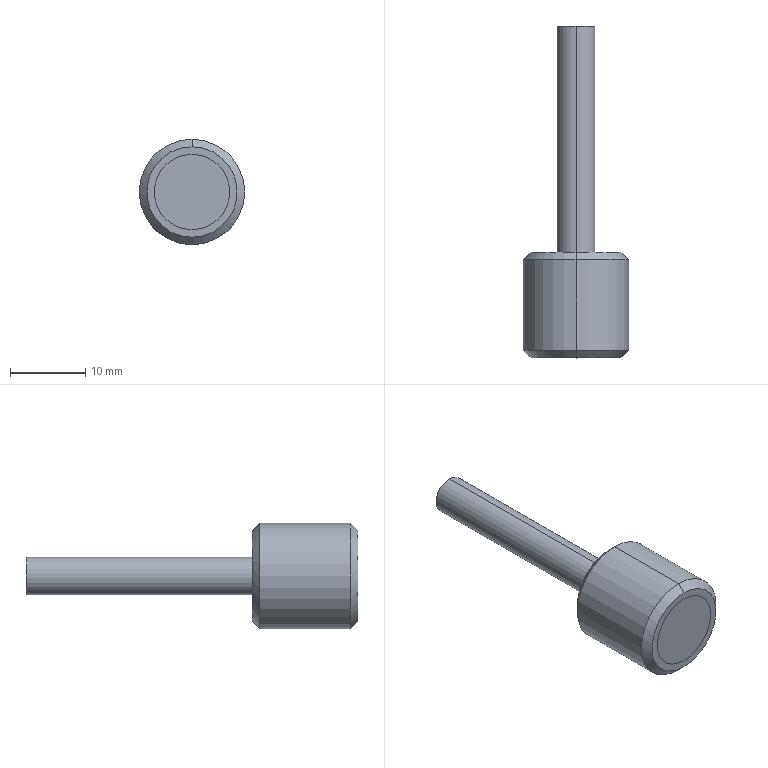Part | STEP file | Pedestal magnet | 2 solids | 18 faces | box 14 x 44 x 14 mm | volume 2702 mm3 | cylinder 8 | plane 6 | cone 4 | commonest cylinder face diameters 10 x4 5 x2 14 x2
STEP:
#1=CARTESIAN_POINT('',(0.,0.,0.));
#2=DIRECTION('',(0.,0.,1.));
#3=DIRECTION('',(1.,0.,0.));
#4=AXIS2_PLACEMENT_3D('',#1,#2,#3);
#5=CARTESIAN_POINT('',(0.,0.,-6.));
#6=VERTEX_POINT('',#5);
#7=CARTESIAN_POINT('',(0.,0.,6.));
#8=VERTEX_POINT('',#7);
#9=CARTESIAN_POINT('',(0.,0.,0.));
#10=DIRECTION('',(0.,-1.,0.));
#11=DIRECTION('',(0.,0.,1.));
#12=AXIS2_PLACEMENT_3D('',#9,#10,#11);
#13=CIRCLE('',#12,6.);
#14=CARTESIAN_POINT('',(0.,1.,0.));
#15=DIRECTION('',(0.,1.,0.));
#16=DIRECTION('',(0.,0.,1.));
#17=AXIS2_PLACEMENT_3D('',#14,#15,#16);
#18=CONICAL_SURFACE('',#17,7.,0.7854);
#19=CARTESIAN_POINT('',(6.283,-1.));
#20=DIRECTION('',(-1.,0.));
#21=VECTOR('',#20,1.);
#22=LINE('',#19,#21);
#23=(GEOMETRIC_REPRESENTATION_CONTEXT(2)PARAMETRIC_REPRESENTATION_CONTEXT()REPRESENTATION_CONTEXT('',''));
#24=DEFINITIONAL_REPRESENTATION('',(#22),#23);
#25=PCURVE('',#18,#24);
#26=CARTESIAN_POINT('',(0.,0.,0.));
#27=DIRECTION('',(0.,1.,0.));
#28=DIRECTION('',(0.,0.,1.));
#29=AXIS2_PLACEMENT_3D('',#26,#27,#28);
#30=PLANE('',#29);
#31=CARTESIAN_POINT('',(6.,0.));
#32=CARTESIAN_POINT('',(6.,-10.392));
#33=CARTESIAN_POINT('',(-3.,-5.196));
#34=CARTESIAN_POINT('',(-12.,0.));
#35=CARTESIAN_POINT('',(-3.,5.196));
#36=CARTESIAN_POINT('',(6.,10.392));
#37=CARTESIAN_POINT('',(6.,0.));
#38=(BOUNDED_CURVE()B_SPLINE_CURVE(2,(#31,#32,#33,#34,#35,#36,#37),.UNSPECIFIED.,.T.,.F.)B_SPLINE_CURVE_WITH_KNOTS((1,2,2,2,2,1),(-2.094,0.,2.094,4.189,6.283,8.378),.UNSPECIFIED.)CURVE()GEOMETRIC_REPRESENTATION_ITEM()RATIONAL_B_SPLINE_CURVE((1.,0.5,1.,0.5,1.,0.5,1.))REPRESENTATION_ITEM(''));
#39=(GEOMETRIC_REPRESENTATION_CONTEXT(2)PARAMETRIC_REPRESENTATION_CONTEXT()REPRESENTATION_CONTEXT('',''));
#40=DEFINITIONAL_REPRESENTATION('',(#38),#39);
#41=PCURVE('',#30,#40);
#42=SURFACE_CURVE('',#13,(#25,#41),.PCURVE_S1.);
#43=EDGE_CURVE('',#6,#8,#42,.T.);
#44=ORIENTED_EDGE('',*,*,#43,.F.);
#45=CARTESIAN_POINT('',(0.,1.,-7.));
#46=VERTEX_POINT('',#45);
#47=CARTESIAN_POINT('',(0.,1.,-7.));
#48=DIRECTION('',(0.,0.7071,-0.7071));
#49=VECTOR('',#48,1.);
#50=LINE('',#47,#49);
#51=CARTESIAN_POINT('',(3.142,0.));
#52=DIRECTION('',(0.,1.));
#53=VECTOR('',#52,1.);
#54=LINE('',#51,#53);
#55=(GEOMETRIC_REPRESENTATION_CONTEXT(2)PARAMETRIC_REPRESENTATION_CONTEXT()REPRESENTATION_CONTEXT('',''));
#56=DEFINITIONAL_REPRESENTATION('',(#54),#55);
#57=PCURVE('',#18,#56);
#58=CARTESIAN_POINT('',(0.,1.,0.));
#59=DIRECTION('',(0.,1.,0.));
#60=DIRECTION('',(0.,0.,1.));
#61=AXIS2_PLACEMENT_3D('',#58,#59,#60);
#62=CONICAL_SURFACE('',#61,7.,0.7854);
#63=CARTESIAN_POINT('',(3.142,0.));
#64=DIRECTION('',(0.,1.));
#65=VECTOR('',#64,1.);
#66=LINE('',#63,#65);
#67=(GEOMETRIC_REPRESENTATION_CONTEXT(2)PARAMETRIC_REPRESENTATION_CONTEXT()REPRESENTATION_CONTEXT('',''));
#68=DEFINITIONAL_REPRESENTATION('',(#66),#67);
#69=PCURVE('',#62,#68);
#70=SURFACE_CURVE('',#50,(#57,#69),.PCURVE_S1.);
#71=EDGE_CURVE('',#6,#46,#70,.T.);
#72=ORIENTED_EDGE('',*,*,#71,.T.);
#73=CARTESIAN_POINT('',(0.,1.,7.));
#74=VERTEX_POINT('',#73);
#75=CARTESIAN_POINT('',(0.,1.,0.));
#76=DIRECTION('',(0.,1.,0.));
#77=DIRECTION('',(0.,0.,1.));
#78=AXIS2_PLACEMENT_3D('',#75,#76,#77);
#79=CIRCLE('',#78,7.);
#80=CARTESIAN_POINT('',(0.,0.));
#81=DIRECTION('',(1.,0.));
#82=VECTOR('',#81,1.);
#83=LINE('',#80,#82);
#84=(GEOMETRIC_REPRESENTATION_CONTEXT(2)PARAMETRIC_REPRESENTATION_CONTEXT()REPRESENTATION_CONTEXT('',''));
#85=DEFINITIONAL_REPRESENTATION('',(#83),#84);
#86=PCURVE('',#18,#85);
#87=CARTESIAN_POINT('',(0.,14.,0.));
#88=DIRECTION('',(0.,-1.,0.));
#89=DIRECTION('',(0.,0.,-1.));
#90=AXIS2_PLACEMENT_3D('',#87,#88,#89);
#91=CYLINDRICAL_SURFACE('',#90,7.);
#92=CARTESIAN_POINT('',(3.142,13.));
#93=DIRECTION('',(-1.,0.));
#94=VECTOR('',#93,1.);
#95=LINE('',#92,#94);
#96=(GEOMETRIC_REPRESENTATION_CONTEXT(2)PARAMETRIC_REPRESENTATION_CONTEXT()REPRESENTATION_CONTEXT('',''));
#97=DEFINITIONAL_REPRESENTATION('',(#95),#96);
#98=PCURVE('',#91,#97);
#99=SURFACE_CURVE('',#79,(#86,#98),.PCURVE_S1.);
#100=EDGE_CURVE('',#74,#46,#99,.T.);
#101=ORIENTED_EDGE('',*,*,#100,.F.);
#102=CARTESIAN_POINT('',(0.,1.,7.));
#103=DIRECTION('',(0.,0.7071,0.7071));
#104=VECTOR('',#103,1.);
#105=LINE('',#102,#104);
#106=CARTESIAN_POINT('',(0.,0.));
#107=DIRECTION('',(0.,1.));
#108=VECTOR('',#107,1.);
#109=LINE('',#106,#108);
#110=(GEOMETRIC_REPRESENTATION_CONTEXT(2)PARAMETRIC_REPRESENTATION_CONTEXT()REPRESENTATION_CONTEXT('',''));
#111=DEFINITIONAL_REPRESENTATION('',(#109),#110);
#112=PCURVE('',#18,#111);
#113=CARTESIAN_POINT('',(6.283,0.));
#114=DIRECTION('',(0.,1.));
#115=VECTOR('',#114,1.);
#116=LINE('',#113,#115);
#117=(GEOMETRIC_REPRESENTATION_CONTEXT(2)PARAMETRIC_REPRESENTATION_CONTEXT()REPRESENTATION_CONTEXT('',''));
#118=DEFINITIONAL_REPRESENTATION('',(#116),#117);
#119=PCURVE('',#62,#118);
#120=SURFACE_CURVE('',#105,(#112,#119),.PCURVE_S1.);
#121=EDGE_CURVE('',#8,#74,#120,.T.);
#122=ORIENTED_EDGE('',*,*,#121,.F.);
#123=EDGE_LOOP('',(#44,#72,#101,#122));
#124=FACE_BOUND('',#123,.T.);
#125=ADVANCED_FACE('',(#124),#18,.T.);
#126=CARTESIAN_POINT('',(0.,14.,6.));
#127=VERTEX_POINT('',#126);
#128=CARTESIAN_POINT('',(0.,14.,-6.));
#129=VERTEX_POINT('',#128);
#130=CARTESIAN_POINT('',(0.,14.,0.));
#131=DIRECTION('',(0.,1.,0.));
#132=DIRECTION('',(0.,0.,1.));
#133=AXIS2_PLACEMENT_3D('',#130,#131,#132);
#134=CIRCLE('',#133,6.);
#135=CARTESIAN_POINT('',(0.,14.,0.));
#136=DIRECTION('',(0.,-1.,0.));
#137=DIRECTION('',(0.,0.,-1.));
#138=AXIS2_PLACEMENT_3D('',#135,#136,#137);
#139=CONICAL_SURFACE('',#138,6.,0.7854);
#140=CARTESIAN_POINT('',(3.142,0.));
#141=DIRECTION('',(-1.,0.));
#142=VECTOR('',#141,1.);
#143=LINE('',#140,#142);
#144=(GEOMETRIC_REPRESENTATION_CONTEXT(2)PARAMETRIC_REPRESENTATION_CONTEXT()REPRESENTATION_CONTEXT('',''));
#145=DEFINITIONAL_REPRESENTATION('',(#143),#144);
#146=PCURVE('',#139,#145);
#147=CARTESIAN_POINT('',(0.,14.,0.));
#148=DIRECTION('',(0.,1.,0.));
#149=DIRECTION('',(0.,0.,1.));
#150=AXIS2_PLACEMENT_3D('',#147,#148,#149);
#151=PLANE('',#150);
#152=CARTESIAN_POINT('',(0.,0.));
#153=DIRECTION('',(1.,0.));
#154=AXIS2_PLACEMENT_2D('',#152,#153);
#155=CIRCLE('',#154,6.);
#156=(GEOMETRIC_REPRESENTATION_CONTEXT(2)PARAMETRIC_REPRESENTATION_CONTEXT()REPRESENTATION_CONTEXT('',''));
#157=DEFINITIONAL_REPRESENTATION('',(#155),#156);
#158=PCURVE('',#151,#157);
#159=SURFACE_CURVE('',#134,(#146,#158),.PCURVE_S1.);
#160=EDGE_CURVE('',#127,#129,#159,.T.);
#161=ORIENTED_EDGE('',*,*,#160,.F.);
#162=CARTESIAN_POINT('',(0.,13.,7.));
#163=VERTEX_POINT('',#162);
#164=CARTESIAN_POINT('',(0.,14.,6.));
#165=DIRECTION('',(0.,-0.7071,0.7071));
#166=VECTOR('',#165,1.);
#167=LINE('',#164,#166);
#168=CARTESIAN_POINT('',(3.142,0.));
#169=DIRECTION('',(0.,1.));
#170=VECTOR('',#169,1.);
#171=LINE('',#168,#170);
#172=(GEOMETRIC_REPRESENTATION_CONTEXT(2)PARAMETRIC_REPRESENTATION_CONTEXT()REPRESENTATION_CONTEXT('',''));
#173=DEFINITIONAL_REPRESENTATION('',(#171),#172);
#174=PCURVE('',#139,#173);
#175=CARTESIAN_POINT('',(0.,14.,0.));
#176=DIRECTION('',(0.,-1.,0.));
#177=DIRECTION('',(0.,0.,-1.));
#178=AXIS2_PLACEMENT_3D('',#175,#176,#177);
#179=CONICAL_SURFACE('',#178,6.,0.7854);
#180=CARTESIAN_POINT('',(3.142,0.));
#181=DIRECTION('',(0.,1.));
#182=VECTOR('',#181,1.);
#183=LINE('',#180,#182);
#184=(GEOMETRIC_REPRESENTATION_CONTEXT(2)PARAMETRIC_REPRESENTATION_CONTEXT()REPRESENTATION_CONTEXT('',''));
#185=DEFINITIONAL_REPRESENTATION('',(#183),#184);
#186=PCURVE('',#179,#185);
#187=SURFACE_CURVE('',#167,(#174,#186),.PCURVE_S1.);
#188=EDGE_CURVE('',#127,#163,#187,.T.);
#189=ORIENTED_EDGE('',*,*,#188,.T.);
#190=CARTESIAN_POINT('',(0.,13.,-7.));
#191=VERTEX_POINT('',#190);
#192=CARTESIAN_POINT('',(0.,13.,0.));
#193=DIRECTION('',(0.,-1.,0.));
#194=DIRECTION('',(0.,0.,1.));
#195=AXIS2_PLACEMENT_3D('',#192,#193,#194);
#196=CIRCLE('',#195,7.);
#197=CARTESIAN_POINT('',(-3.142,1.));
#198=DIRECTION('',(1.,0.));
#199=VECTOR('',#198,1.);
#200=LINE('',#197,#199);
#201=(GEOMETRIC_REPRESENTATION_CONTEXT(2)PARAMETRIC_REPRESENTATION_CONTEXT()REPRESENTATION_CONTEXT('',''));
#202=DEFINITIONAL_REPRESENTATION('',(#200),#201);
#203=PCURVE('',#139,#202);
#204=CARTESIAN_POINT('',(-3.142,1.));
#205=DIRECTION('',(1.,0.));
#206=VECTOR('',#205,1.);
#207=LINE('',#204,#206);
#208=(GEOMETRIC_REPRESENTATION_CONTEXT(2)PARAMETRIC_REPRESENTATION_CONTEXT()REPRESENTATION_CONTEXT('',''));
#209=DEFINITIONAL_REPRESENTATION('',(#207),#208);
#210=PCURVE('',#91,#209);
#211=SURFACE_CURVE('',#196,(#203,#210),.PCURVE_S1.);
#212=EDGE_CURVE('',#191,#163,#211,.T.);
#213=ORIENTED_EDGE('',*,*,#212,.F.);
#214=CARTESIAN_POINT('',(0.,14.,-6.));
#215=DIRECTION('',(0.,-0.7071,-0.7071));
#216=VECTOR('',#215,1.);
#217=LINE('',#214,#216);
#218=CARTESIAN_POINT('',(0.,0.));
#219=DIRECTION('',(0.,1.));
#220=VECTOR('',#219,1.);
#221=LINE('',#218,#220);
#222=(GEOMETRIC_REPRESENTATION_CONTEXT(2)PARAMETRIC_REPRESENTATION_CONTEXT()REPRESENTATION_CONTEXT('',''));
#223=DEFINITIONAL_REPRESENTATION('',(#221),#222);
#224=PCURVE('',#139,#223);
#225=CARTESIAN_POINT('',(6.283,0.));
#226=DIRECTION('',(0.,1.));
#227=VECTOR('',#226,1.);
#228=LINE('',#225,#227);
#229=(GEOMETRIC_REPRESENTATION_CONTEXT(2)PARAMETRIC_REPRESENTATION_CONTEXT()REPRESENTATION_CONTEXT('',''));
#230=DEFINITIONAL_REPRESENTATION('',(#228),#229);
#231=PCURVE('',#179,#230);
#232=SURFACE_CURVE('',#217,(#224,#231),.PCURVE_S1.);
#233=EDGE_CURVE('',#129,#191,#232,.T.);
#234=ORIENTED_EDGE('',*,*,#233,.F.);
#235=EDGE_LOOP('',(#161,#189,#213,#234));
#236=FACE_BOUND('',#235,.T.);
#237=ADVANCED_FACE('',(#236),#139,.T.);
#238=CARTESIAN_POINT('',(0.,44.,2.5));
#239=VERTEX_POINT('',#238);
#240=CARTESIAN_POINT('',(0.,44.,-2.5));
#241=VERTEX_POINT('',#240);
#242=CARTESIAN_POINT('',(0.,44.,0.));
#243=DIRECTION('',(0.,1.,0.));
#244=DIRECTION('',(0.,0.,1.));
#245=AXIS2_PLACEMENT_3D('',#242,#243,#244);
#246=CIRCLE('',#245,2.5);
#247=CARTESIAN_POINT('',(0.,44.,0.));
#248=DIRECTION('',(0.,-1.,0.));
#249=DIRECTION('',(0.,0.,-1.));
#250=AXIS2_PLACEMENT_3D('',#247,#248,#249);
#251=CYLINDRICAL_SURFACE('',#250,2.5);
#252=CARTESIAN_POINT('',(3.142,0.));
#253=DIRECTION('',(-1.,0.));
#254=VECTOR('',#253,1.);
#255=LINE('',#252,#254);
#256=(GEOMETRIC_REPRESENTATION_CONTEXT(2)PARAMETRIC_REPRESENTATION_CONTEXT()REPRESENTATION_CONTEXT('',''));
#257=DEFINITIONAL_REPRESENTATION('',(#255),#256);
#258=PCURVE('',#251,#257);
#259=CARTESIAN_POINT('',(0.,44.,0.));
#260=DIRECTION('',(0.,1.,0.));
#261=DIRECTION('',(0.,0.,1.));
#262=AXIS2_PLACEMENT_3D('',#259,#260,#261);
#263=PLANE('',#262);
#264=CARTESIAN_POINT('',(0.,0.));
#265=DIRECTION('',(1.,0.));
#266=AXIS2_PLACEMENT_2D('',#264,#265);
#267=CIRCLE('',#266,2.5);
#268=(GEOMETRIC_REPRESENTATION_CONTEXT(2)PARAMETRIC_REPRESENTATION_CONTEXT()REPRESENTATION_CONTEXT('',''));
#269=DEFINITIONAL_REPRESENTATION('',(#267),#268);
#270=PCURVE('',#263,#269);
#271=SURFACE_CURVE('',#246,(#258,#270),.PCURVE_S1.);
#272=EDGE_CURVE('',#239,#241,#271,.T.);
#273=ORIENTED_EDGE('',*,*,#272,.F.);
#274=CARTESIAN_POINT('',(0.,14.,2.5));
#275=VERTEX_POINT('',#274);
#276=CARTESIAN_POINT('',(0.,44.,2.5));
#277=DIRECTION('',(0.,-1.,0.));
#278=VECTOR('',#277,1.);
#279=LINE('',#276,#278);
#280=CARTESIAN_POINT('',(3.142,0.));
#281=DIRECTION('',(0.,1.));
#282=VECTOR('',#281,1.);
#283=LINE('',#280,#282);
#284=(GEOMETRIC_REPRESENTATION_CONTEXT(2)PARAMETRIC_REPRESENTATION_CONTEXT()REPRESENTATION_CONTEXT('',''));
#285=DEFINITIONAL_REPRESENTATION('',(#283),#284);
#286=PCURVE('',#251,#285);
#287=CARTESIAN_POINT('',(0.,44.,0.));
#288=DIRECTION('',(0.,-1.,0.));
#289=DIRECTION('',(0.,0.,-1.));
#290=AXIS2_PLACEMENT_3D('',#287,#288,#289);
#291=CYLINDRICAL_SURFACE('',#290,2.5);
#292=CARTESIAN_POINT('',(3.142,0.));
#293=DIRECTION('',(0.,1.));
#294=VECTOR('',#293,1.);
#295=LINE('',#292,#294);
#296=(GEOMETRIC_REPRESENTATION_CONTEXT(2)PARAMETRIC_REPRESENTATION_CONTEXT()REPRESENTATION_CONTEXT('',''));
#297=DEFINITIONAL_REPRESENTATION('',(#295),#296);
#298=PCURVE('',#291,#297);
#299=SURFACE_CURVE('',#279,(#286,#298),.PCURVE_S1.);
#300=EDGE_CURVE('',#239,#275,#299,.T.);
#301=ORIENTED_EDGE('',*,*,#300,.T.);
#302=CARTESIAN_POINT('',(0.,14.,-2.5));
#303=VERTEX_POINT('',#302);
#304=CARTESIAN_POINT('',(0.,14.,0.));
#305=DIRECTION('',(0.,1.,0.));
#306=DIRECTION('',(0.,0.,1.));
#307=AXIS2_PLACEMENT_3D('',#304,#305,#306);
#308=CIRCLE('',#307,2.5);
#309=CARTESIAN_POINT('',(3.142,30.));
#310=DIRECTION('',(-1.,0.));
#311=VECTOR('',#310,1.);
#312=LINE('',#309,#311);
#313=(GEOMETRIC_REPRESENTATION_CONTEXT(2)PARAMETRIC_REPRESENTATION_CONTEXT()REPRESENTATION_CONTEXT('',''));
#314=DEFINITIONAL_REPRESENTATION('',(#312),#313);
#315=PCURVE('',#251,#314);
#316=CARTESIAN_POINT('',(0.,0.));
#317=DIRECTION('',(1.,0.));
#318=AXIS2_PLACEMENT_2D('',#316,#317);
#319=CIRCLE('',#318,2.5);
#320=(GEOMETRIC_REPRESENTATION_CONTEXT(2)PARAMETRIC_REPRESENTATION_CONTEXT()REPRESENTATION_CONTEXT('',''));
#321=DEFINITIONAL_REPRESENTATION('',(#319),#320);
#322=PCURVE('',#151,#321);
#323=SURFACE_CURVE('',#308,(#315,#322),.PCURVE_S1.);
#324=EDGE_CURVE('',#275,#303,#323,.T.);
#325=ORIENTED_EDGE('',*,*,#324,.T.);
#326=CARTESIAN_POINT('',(0.,44.,-2.5));
#327=DIRECTION('',(0.,-1.,0.));
#328=VECTOR('',#327,1.);
#329=LINE('',#326,#328);
#330=CARTESIAN_POINT('',(0.,0.));
#331=DIRECTION('',(0.,1.));
#332=VECTOR('',#331,1.);
#333=LINE('',#330,#332);
#334=(GEOMETRIC_REPRESENTATION_CONTEXT(2)PARAMETRIC_REPRESENTATION_CONTEXT()REPRESENTATION_CONTEXT('',''));
#335=DEFINITIONAL_REPRESENTATION('',(#333),#334);
#336=PCURVE('',#251,#335);
#337=CARTESIAN_POINT('',(6.283,0.));
#338=DIRECTION('',(0.,1.));
#339=VECTOR('',#338,1.);
#340=LINE('',#337,#339);
#341=(GEOMETRIC_REPRESENTATION_CONTEXT(2)PARAMETRIC_REPRESENTATION_CONTEXT()REPRESENTATION_CONTEXT('',''));
#342=DEFINITIONAL_REPRESENTATION('',(#340),#341);
#343=PCURVE('',#291,#342);
#344=SURFACE_CURVE('',#329,(#336,#343),.PCURVE_S1.);
#345=EDGE_CURVE('',#241,#303,#344,.T.);
#346=ORIENTED_EDGE('',*,*,#345,.F.);
#347=EDGE_LOOP('',(#273,#301,#325,#346));
#348=FACE_BOUND('',#347,.T.);
#349=ADVANCED_FACE('',(#348),#251,.T.);
#350=CARTESIAN_POINT('',(0.,5.,-5.));
#351=VERTEX_POINT('',#350);
#352=CARTESIAN_POINT('',(0.,0.,-5.));
#353=VERTEX_POINT('',#352);
#354=CARTESIAN_POINT('',(0.,5.,-5.));
#355=DIRECTION('',(0.,-1.,0.));
#356=VECTOR('',#355,1.);
#357=LINE('',#354,#356);
#358=CARTESIAN_POINT('',(0.,5.,0.));
#359=DIRECTION('',(0.,-1.,0.));
#360=DIRECTION('',(0.,0.,-1.));
#361=AXIS2_PLACEMENT_3D('',#358,#359,#360);
#362=CYLINDRICAL_SURFACE('',#361,5.);
#363=CARTESIAN_POINT('',(6.283,0.));
#364=DIRECTION('',(0.,1.));
#365=VECTOR('',#364,1.);
#366=LINE('',#363,#365);
#367=(GEOMETRIC_REPRESENTATION_CONTEXT(2)PARAMETRIC_REPRESENTATION_CONTEXT()REPRESENTATION_CONTEXT('',''));
#368=DEFINITIONAL_REPRESENTATION('',(#366),#367);
#369=PCURVE('',#362,#368);
#370=CARTESIAN_POINT('',(0.,5.,0.));
#371=DIRECTION('',(0.,-1.,0.));
#372=DIRECTION('',(0.,0.,-1.));
#373=AXIS2_PLACEMENT_3D('',#370,#371,#372);
#374=CYLINDRICAL_SURFACE('',#373,5.);
#375=CARTESIAN_POINT('',(0.,0.));
#376=DIRECTION('',(0.,1.));
#377=VECTOR('',#376,1.);
#378=LINE('',#375,#377);
#379=(GEOMETRIC_REPRESENTATION_CONTEXT(2)PARAMETRIC_REPRESENTATION_CONTEXT()REPRESENTATION_CONTEXT('',''));
#380=DEFINITIONAL_REPRESENTATION('',(#378),#379);
#381=PCURVE('',#374,#380);
#382=SURFACE_CURVE('',#357,(#369,#381),.PCURVE_S1.);
#383=EDGE_CURVE('',#351,#353,#382,.T.);
#384=ORIENTED_EDGE('',*,*,#383,.T.);
#385=CARTESIAN_POINT('',(0.,0.,5.));
#386=VERTEX_POINT('',#385);
#387=CARTESIAN_POINT('',(0.,0.,0.));
#388=DIRECTION('',(0.,1.,0.));
#389=DIRECTION('',(0.,0.,1.));
#390=AXIS2_PLACEMENT_3D('',#387,#388,#389);
#391=CIRCLE('',#390,5.);
#392=CARTESIAN_POINT('',(9.425,5.));
#393=DIRECTION('',(-1.,0.));
#394=VECTOR('',#393,1.);
#395=LINE('',#392,#394);
#396=(GEOMETRIC_REPRESENTATION_CONTEXT(2)PARAMETRIC_REPRESENTATION_CONTEXT()REPRESENTATION_CONTEXT('',''));
#397=DEFINITIONAL_REPRESENTATION('',(#395),#396);
#398=PCURVE('',#362,#397);
#399=CARTESIAN_POINT('',(0.,0.));
#400=DIRECTION('',(1.,0.));
#401=AXIS2_PLACEMENT_2D('',#399,#400);
#402=CIRCLE('',#401,5.);
#403=(GEOMETRIC_REPRESENTATION_CONTEXT(2)PARAMETRIC_REPRESENTATION_CONTEXT()REPRESENTATION_CONTEXT('',''));
#404=DEFINITIONAL_REPRESENTATION('',(#402),#403);
#405=PCURVE('',#30,#404);
#406=SURFACE_CURVE('',#391,(#398,#405),.PCURVE_S1.);
#407=EDGE_CURVE('',#353,#386,#406,.T.);
#408=ORIENTED_EDGE('',*,*,#407,.T.);
#409=CARTESIAN_POINT('',(0.,5.,5.));
#410=VERTEX_POINT('',#409);
#411=CARTESIAN_POINT('',(0.,5.,5.));
#412=DIRECTION('',(0.,-1.,0.));
#413=VECTOR('',#412,1.);
#414=LINE('',#411,#413);
#415=CARTESIAN_POINT('',(3.142,0.));
#416=DIRECTION('',(0.,1.));
#417=VECTOR('',#416,1.);
#418=LINE('',#415,#417);
#419=(GEOMETRIC_REPRESENTATION_CONTEXT(2)PARAMETRIC_REPRESENTATION_CONTEXT()REPRESENTATION_CONTEXT('',''));
#420=DEFINITIONAL_REPRESENTATION('',(#418),#419);
#421=PCURVE('',#362,#420);
#422=CARTESIAN_POINT('',(3.142,0.));
#423=DIRECTION('',(0.,1.));
#424=VECTOR('',#423,1.);
#425=LINE('',#422,#424);
#426=(GEOMETRIC_REPRESENTATION_CONTEXT(2)PARAMETRIC_REPRESENTATION_CONTEXT()REPRESENTATION_CONTEXT('',''));
#427=DEFINITIONAL_REPRESENTATION('',(#425),#426);
#428=PCURVE('',#374,#427);
#429=SURFACE_CURVE('',#414,(#421,#428),.PCURVE_S1.);
#430=EDGE_CURVE('',#410,#386,#429,.T.);
#431=ORIENTED_EDGE('',*,*,#430,.F.);
#432=CARTESIAN_POINT('',(0.,5.,0.));
#433=DIRECTION('',(0.,1.,0.));
#434=DIRECTION('',(0.,0.,1.));
#435=AXIS2_PLACEMENT_3D('',#432,#433,#434);
#436=CIRCLE('',#435,5.);
#437=CARTESIAN_POINT('',(9.425,0.));
#438=DIRECTION('',(-1.,0.));
#439=VECTOR('',#438,1.);
#440=LINE('',#437,#439);
#441=(GEOMETRIC_REPRESENTATION_CONTEXT(2)PARAMETRIC_REPRESENTATION_CONTEXT()REPRESENTATION_CONTEXT('',''));
#442=DEFINITIONAL_REPRESENTATION('',(#440),#441);
#443=PCURVE('',#362,#442);
#444=CARTESIAN_POINT('',(0.,5.,0.));
#445=DIRECTION('',(0.,1.,0.));
#446=DIRECTION('',(0.,0.,1.));
#447=AXIS2_PLACEMENT_3D('',#444,#445,#446);
#448=PLANE('',#447);
#449=CARTESIAN_POINT('',(0.,0.));
#450=DIRECTION('',(1.,0.));
#451=AXIS2_PLACEMENT_2D('',#449,#450);
#452=CIRCLE('',#451,5.);
#453=(GEOMETRIC_REPRESENTATION_CONTEXT(2)PARAMETRIC_REPRESENTATION_CONTEXT()REPRESENTATION_CONTEXT('',''));
#454=DEFINITIONAL_REPRESENTATION('',(#452),#453);
#455=PCURVE('',#448,#454);
#456=SURFACE_CURVE('',#436,(#443,#455),.PCURVE_S1.);
#457=EDGE_CURVE('',#351,#410,#456,.T.);
#458=ORIENTED_EDGE('',*,*,#457,.F.);
#459=EDGE_LOOP('',(#384,#408,#431,#458));
#460=FACE_BOUND('',#459,.F.);
#461=ADVANCED_FACE('',(#460),#362,.F.);
#462=ORIENTED_EDGE('',*,*,#212,.T.);
#463=CARTESIAN_POINT('',(0.,14.,7.));
#464=DIRECTION('',(0.,-1.,0.));
#465=VECTOR('',#464,1.);
#466=LINE('',#463,#465);
#467=CARTESIAN_POINT('',(3.142,0.));
#468=DIRECTION('',(0.,1.));
#469=VECTOR('',#468,1.);
#470=LINE('',#467,#469);
#471=(GEOMETRIC_REPRESENTATION_CONTEXT(2)PARAMETRIC_REPRESENTATION_CONTEXT()REPRESENTATION_CONTEXT('',''));
#472=DEFINITIONAL_REPRESENTATION('',(#470),#471);
#473=PCURVE('',#91,#472);
#474=CARTESIAN_POINT('',(0.,14.,0.));
#475=DIRECTION('',(0.,-1.,0.));
#476=DIRECTION('',(0.,0.,-1.));
#477=AXIS2_PLACEMENT_3D('',#474,#475,#476);
#478=CYLINDRICAL_SURFACE('',#477,7.);
#479=CARTESIAN_POINT('',(3.142,0.));
#480=DIRECTION('',(0.,1.));
#481=VECTOR('',#480,1.);
#482=LINE('',#479,#481);
#483=(GEOMETRIC_REPRESENTATION_CONTEXT(2)PARAMETRIC_REPRESENTATION_CONTEXT()REPRESENTATION_CONTEXT('',''));
#484=DEFINITIONAL_REPRESENTATION('',(#482),#483);
#485=PCURVE('',#478,#484);
#486=SURFACE_CURVE('',#466,(#473,#485),.PCURVE_S1.);
#487=EDGE_CURVE('',#163,#74,#486,.T.);
#488=ORIENTED_EDGE('',*,*,#487,.T.);
#489=ORIENTED_EDGE('',*,*,#100,.T.);
#490=CARTESIAN_POINT('',(0.,14.,-7.));
#491=DIRECTION('',(0.,-1.,0.));
#492=VECTOR('',#491,1.);
#493=LINE('',#490,#492);
#494=CARTESIAN_POINT('',(0.,0.));
#495=DIRECTION('',(0.,1.));
#496=VECTOR('',#495,1.);
#497=LINE('',#494,#496);
#498=(GEOMETRIC_REPRESENTATION_CONTEXT(2)PARAMETRIC_REPRESENTATION_CONTEXT()REPRESENTATION_CONTEXT('',''));
#499=DEFINITIONAL_REPRESENTATION('',(#497),#498);
#500=PCURVE('',#91,#499);
#501=CARTESIAN_POINT('',(6.283,0.));
#502=DIRECTION('',(0.,1.));
#503=VECTOR('',#502,1.);
#504=LINE('',#501,#503);
#505=(GEOMETRIC_REPRESENTATION_CONTEXT(2)PARAMETRIC_REPRESENTATION_CONTEXT()REPRESENTATION_CONTEXT('',''));
#506=DEFINITIONAL_REPRESENTATION('',(#504),#505);
#507=PCURVE('',#478,#506);
#508=SURFACE_CURVE('',#493,(#500,#507),.PCURVE_S1.);
#509=EDGE_CURVE('',#191,#46,#508,.T.);
#510=ORIENTED_EDGE('',*,*,#509,.F.);
#511=EDGE_LOOP('',(#462,#488,#489,#510));
#512=FACE_BOUND('',#511,.T.);
#513=ADVANCED_FACE('',(#512),#91,.T.);
#514=ORIENTED_EDGE('',*,*,#487,.F.);
#515=CARTESIAN_POINT('',(0.,13.,0.));
#516=DIRECTION('',(0.,-1.,0.));
#517=DIRECTION('',(0.,0.,1.));
#518=AXIS2_PLACEMENT_3D('',#515,#516,#517);
#519=CIRCLE('',#518,7.);
#520=CARTESIAN_POINT('',(3.142,1.));
#521=DIRECTION('',(1.,0.));
#522=VECTOR('',#521,1.);
#523=LINE('',#520,#522);
#524=(GEOMETRIC_REPRESENTATION_CONTEXT(2)PARAMETRIC_REPRESENTATION_CONTEXT()REPRESENTATION_CONTEXT('',''));
#525=DEFINITIONAL_REPRESENTATION('',(#523),#524);
#526=PCURVE('',#478,#525);
#527=CARTESIAN_POINT('',(3.142,1.));
#528=DIRECTION('',(1.,0.));
#529=VECTOR('',#528,1.);
#530=LINE('',#527,#529);
#531=(GEOMETRIC_REPRESENTATION_CONTEXT(2)PARAMETRIC_REPRESENTATION_CONTEXT()REPRESENTATION_CONTEXT('',''));
#532=DEFINITIONAL_REPRESENTATION('',(#530),#531);
#533=PCURVE('',#179,#532);
#534=SURFACE_CURVE('',#519,(#526,#533),.PCURVE_S1.);
#535=EDGE_CURVE('',#163,#191,#534,.T.);
#536=ORIENTED_EDGE('',*,*,#535,.T.);
#537=ORIENTED_EDGE('',*,*,#509,.T.);
#538=CARTESIAN_POINT('',(0.,1.,0.));
#539=DIRECTION('',(0.,1.,0.));
#540=DIRECTION('',(0.,0.,1.));
#541=AXIS2_PLACEMENT_3D('',#538,#539,#540);
#542=CIRCLE('',#541,7.);
#543=CARTESIAN_POINT('',(9.425,13.));
#544=DIRECTION('',(-1.,0.));
#545=VECTOR('',#544,1.);
#546=LINE('',#543,#545);
#547=(GEOMETRIC_REPRESENTATION_CONTEXT(2)PARAMETRIC_REPRESENTATION_CONTEXT()REPRESENTATION_CONTEXT('',''));
#548=DEFINITIONAL_REPRESENTATION('',(#546),#547);
#549=PCURVE('',#478,#548);
#550=CARTESIAN_POINT('',(0.,0.));
#551=DIRECTION('',(1.,0.));
#552=VECTOR('',#551,1.);
#553=LINE('',#550,#552);
#554=(GEOMETRIC_REPRESENTATION_CONTEXT(2)PARAMETRIC_REPRESENTATION_CONTEXT()REPRESENTATION_CONTEXT('',''));
#555=DEFINITIONAL_REPRESENTATION('',(#553),#554);
#556=PCURVE('',#62,#555);
#557=SURFACE_CURVE('',#542,(#549,#556),.PCURVE_S1.);
#558=EDGE_CURVE('',#46,#74,#557,.T.);
#559=ORIENTED_EDGE('',*,*,#558,.T.);
#560=EDGE_LOOP('',(#514,#536,#537,#559));
#561=FACE_BOUND('',#560,.T.);
#562=ADVANCED_FACE('',(#561),#478,.T.);
#563=CARTESIAN_POINT('',(0.,14.,0.));
#564=DIRECTION('',(0.,1.,0.));
#565=DIRECTION('',(0.,0.,1.));
#566=AXIS2_PLACEMENT_3D('',#563,#564,#565);
#567=CIRCLE('',#566,6.);
#568=CARTESIAN_POINT('',(0.,0.));
#569=DIRECTION('',(1.,0.));
#570=AXIS2_PLACEMENT_2D('',#568,#569);
#571=CIRCLE('',#570,6.);
#572=(GEOMETRIC_REPRESENTATION_CONTEXT(2)PARAMETRIC_REPRESENTATION_CONTEXT()REPRESENTATION_CONTEXT('',''));
#573=DEFINITIONAL_REPRESENTATION('',(#571),#572);
#574=PCURVE('',#151,#573);
#575=CARTESIAN_POINT('',(9.425,0.));
#576=DIRECTION('',(-1.,0.));
#577=VECTOR('',#576,1.);
#578=LINE('',#575,#577);
#579=(GEOMETRIC_REPRESENTATION_CONTEXT(2)PARAMETRIC_REPRESENTATION_CONTEXT()REPRESENTATION_CONTEXT('',''));
#580=DEFINITIONAL_REPRESENTATION('',(#578),#579);
#581=PCURVE('',#179,#580);
#582=SURFACE_CURVE('',#567,(#574,#581),.PCURVE_S1.);
#583=EDGE_CURVE('',#129,#127,#582,.T.);
#584=ORIENTED_EDGE('',*,*,#583,.T.);
#585=ORIENTED_EDGE('',*,*,#160,.T.);
#586=EDGE_LOOP('',(#584,#585));
#587=FACE_BOUND('',#586,.T.);
#588=CARTESIAN_POINT('',(0.,14.,0.));
#589=DIRECTION('',(0.,1.,0.));
#590=DIRECTION('',(0.,0.,1.));
#591=AXIS2_PLACEMENT_3D('',#588,#589,#590);
#592=CIRCLE('',#591,2.5);
#593=CARTESIAN_POINT('',(0.,0.));
#594=DIRECTION('',(1.,0.));
#595=AXIS2_PLACEMENT_2D('',#593,#594);
#596=CIRCLE('',#595,2.5);
#597=(GEOMETRIC_REPRESENTATION_CONTEXT(2)PARAMETRIC_REPRESENTATION_CONTEXT()REPRESENTATION_CONTEXT('',''));
#598=DEFINITIONAL_REPRESENTATION('',(#596),#597);
#599=PCURVE('',#151,#598);
#600=CARTESIAN_POINT('',(9.425,30.));
#601=DIRECTION('',(-1.,0.));
#602=VECTOR('',#601,1.);
#603=LINE('',#600,#602);
#604=(GEOMETRIC_REPRESENTATION_CONTEXT(2)PARAMETRIC_REPRESENTATION_CONTEXT()REPRESENTATION_CONTEXT('',''));
#605=DEFINITIONAL_REPRESENTATION('',(#603),#604);
#606=PCURVE('',#291,#605);
#607=SURFACE_CURVE('',#592,(#599,#606),.PCURVE_S1.);
#608=EDGE_CURVE('',#303,#275,#607,.T.);
#609=ORIENTED_EDGE('',*,*,#608,.F.);
#610=ORIENTED_EDGE('',*,*,#324,.F.);
#611=EDGE_LOOP('',(#609,#610));
#612=FACE_BOUND('',#611,.T.);
#613=ADVANCED_FACE('',(#587,#612),#151,.T.);
#614=CARTESIAN_POINT('',(0.,0.,0.));
#615=DIRECTION('',(0.,-1.,0.));
#616=DIRECTION('',(0.,0.,1.));
#617=AXIS2_PLACEMENT_3D('',#614,#615,#616);
#618=CIRCLE('',#617,6.);
#619=CARTESIAN_POINT('',(6.,0.));
#620=CARTESIAN_POINT('',(6.,-10.392));
#621=CARTESIAN_POINT('',(-3.,-5.196));
#622=CARTESIAN_POINT('',(-12.,0.));
#623=CARTESIAN_POINT('',(-3.,5.196));
#624=CARTESIAN_POINT('',(6.,10.392));
#625=CARTESIAN_POINT('',(6.,0.));
#626=(BOUNDED_CURVE()B_SPLINE_CURVE(2,(#619,#620,#621,#622,#623,#624,#625),.UNSPECIFIED.,.T.,.F.)B_SPLINE_CURVE_WITH_KNOTS((1,2,2,2,2,1),(-2.094,0.,2.094,4.189,6.283,8.378),.UNSPECIFIED.)CURVE()GEOMETRIC_REPRESENTATION_ITEM()RATIONAL_B_SPLINE_CURVE((1.,0.5,1.,0.5,1.,0.5,1.))REPRESENTATION_ITEM(''));
#627=(GEOMETRIC_REPRESENTATION_CONTEXT(2)PARAMETRIC_REPRESENTATION_CONTEXT()REPRESENTATION_CONTEXT('',''));
#628=DEFINITIONAL_REPRESENTATION('',(#626),#627);
#629=PCURVE('',#30,#628);
#630=CARTESIAN_POINT('',(6.283,-1.));
#631=DIRECTION('',(-1.,0.));
#632=VECTOR('',#631,1.);
#633=LINE('',#630,#632);
#634=(GEOMETRIC_REPRESENTATION_CONTEXT(2)PARAMETRIC_REPRESENTATION_CONTEXT()REPRESENTATION_CONTEXT('',''));
#635=DEFINITIONAL_REPRESENTATION('',(#633),#634);
#636=PCURVE('',#62,#635);
#637=SURFACE_CURVE('',#618,(#629,#636),.PCURVE_S1.);
#638=EDGE_CURVE('',#8,#6,#637,.T.);
#639=ORIENTED_EDGE('',*,*,#638,.T.);
#640=ORIENTED_EDGE('',*,*,#43,.T.);
#641=EDGE_LOOP('',(#639,#640));
#642=FACE_BOUND('',#641,.T.);
#643=ORIENTED_EDGE('',*,*,#407,.T.);
#644=CARTESIAN_POINT('',(0.,0.,0.));
#645=DIRECTION('',(0.,1.,0.));
#646=DIRECTION('',(0.,0.,1.));
#647=AXIS2_PLACEMENT_3D('',#644,#645,#646);
#648=CIRCLE('',#647,5.);
#649=CARTESIAN_POINT('',(0.,0.));
#650=DIRECTION('',(1.,0.));
#651=AXIS2_PLACEMENT_2D('',#649,#650);
#652=CIRCLE('',#651,5.);
#653=(GEOMETRIC_REPRESENTATION_CONTEXT(2)PARAMETRIC_REPRESENTATION_CONTEXT()REPRESENTATION_CONTEXT('',''));
#654=DEFINITIONAL_REPRESENTATION('',(#652),#653);
#655=PCURVE('',#30,#654);
#656=CARTESIAN_POINT('',(3.142,5.));
#657=DIRECTION('',(-1.,0.));
#658=VECTOR('',#657,1.);
#659=LINE('',#656,#658);
#660=(GEOMETRIC_REPRESENTATION_CONTEXT(2)PARAMETRIC_REPRESENTATION_CONTEXT()REPRESENTATION_CONTEXT('',''));
#661=DEFINITIONAL_REPRESENTATION('',(#659),#660);
#662=PCURVE('',#374,#661);
#663=SURFACE_CURVE('',#648,(#655,#662),.PCURVE_S1.);
#664=EDGE_CURVE('',#386,#353,#663,.T.);
#665=ORIENTED_EDGE('',*,*,#664,.T.);
#666=EDGE_LOOP('',(#643,#665));
#667=FACE_BOUND('',#666,.T.);
#668=ADVANCED_FACE('',(#642,#667),#30,.F.);
#669=ORIENTED_EDGE('',*,*,#664,.T.);
#670=ORIENTED_EDGE('',*,*,#383,.F.);
#671=CARTESIAN_POINT('',(0.,5.,0.));
#672=DIRECTION('',(0.,1.,0.));
#673=DIRECTION('',(0.,0.,1.));
#674=AXIS2_PLACEMENT_3D('',#671,#672,#673);
#675=CIRCLE('',#674,5.);
#676=CARTESIAN_POINT('',(3.142,0.));
#677=DIRECTION('',(-1.,0.));
#678=VECTOR('',#677,1.);
#679=LINE('',#676,#678);
#680=(GEOMETRIC_REPRESENTATION_CONTEXT(2)PARAMETRIC_REPRESENTATION_CONTEXT()REPRESENTATION_CONTEXT('',''));
#681=DEFINITIONAL_REPRESENTATION('',(#679),#680);
#682=PCURVE('',#374,#681);
#683=CARTESIAN_POINT('',(0.,0.));
#684=DIRECTION('',(1.,0.));
#685=AXIS2_PLACEMENT_2D('',#683,#684);
#686=CIRCLE('',#685,5.);
#687=(GEOMETRIC_REPRESENTATION_CONTEXT(2)PARAMETRIC_REPRESENTATION_CONTEXT()REPRESENTATION_CONTEXT('',''));
#688=DEFINITIONAL_REPRESENTATION('',(#686),#687);
#689=PCURVE('',#448,#688);
#690=SURFACE_CURVE('',#675,(#682,#689),.PCURVE_S1.);
#691=EDGE_CURVE('',#410,#351,#690,.T.);
#692=ORIENTED_EDGE('',*,*,#691,.F.);
#693=ORIENTED_EDGE('',*,*,#430,.T.);
#694=EDGE_LOOP('',(#669,#670,#692,#693));
#695=FACE_BOUND('',#694,.F.);
#696=ADVANCED_FACE('',(#695),#374,.F.);
#697=ORIENTED_EDGE('',*,*,#457,.F.);
#698=ORIENTED_EDGE('',*,*,#691,.F.);
#699=EDGE_LOOP('',(#697,#698));
#700=FACE_BOUND('',#699,.T.);
#701=ADVANCED_FACE('',(#700),#448,.F.);
#702=ORIENTED_EDGE('',*,*,#300,.F.);
#703=CARTESIAN_POINT('',(0.,44.,0.));
#704=DIRECTION('',(0.,1.,0.));
#705=DIRECTION('',(0.,0.,1.));
#706=AXIS2_PLACEMENT_3D('',#703,#704,#705);
#707=CIRCLE('',#706,2.5);
#708=CARTESIAN_POINT('',(9.425,0.));
#709=DIRECTION('',(-1.,0.));
#710=VECTOR('',#709,1.);
#711=LINE('',#708,#710);
#712=(GEOMETRIC_REPRESENTATION_CONTEXT(2)PARAMETRIC_REPRESENTATION_CONTEXT()REPRESENTATION_CONTEXT('',''));
#713=DEFINITIONAL_REPRESENTATION('',(#711),#712);
#714=PCURVE('',#291,#713);
#715=CARTESIAN_POINT('',(0.,0.));
#716=DIRECTION('',(1.,0.));
#717=AXIS2_PLACEMENT_2D('',#715,#716);
#718=CIRCLE('',#717,2.5);
#719=(GEOMETRIC_REPRESENTATION_CONTEXT(2)PARAMETRIC_REPRESENTATION_CONTEXT()REPRESENTATION_CONTEXT('',''));
#720=DEFINITIONAL_REPRESENTATION('',(#718),#719);
#721=PCURVE('',#263,#720);
#722=SURFACE_CURVE('',#707,(#714,#721),.PCURVE_S1.);
#723=EDGE_CURVE('',#241,#239,#722,.T.);
#724=ORIENTED_EDGE('',*,*,#723,.F.);
#725=ORIENTED_EDGE('',*,*,#345,.T.);
#726=ORIENTED_EDGE('',*,*,#608,.T.);
#727=EDGE_LOOP('',(#702,#724,#725,#726));
#728=FACE_BOUND('',#727,.T.);
#729=ADVANCED_FACE('',(#728),#291,.T.);
#730=ORIENTED_EDGE('',*,*,#723,.T.);
#731=ORIENTED_EDGE('',*,*,#272,.T.);
#732=EDGE_LOOP('',(#730,#731));
#733=FACE_BOUND('',#732,.T.);
#734=ADVANCED_FACE('',(#733),#263,.T.);
#735=ORIENTED_EDGE('',*,*,#188,.F.);
#736=ORIENTED_EDGE('',*,*,#583,.F.);
#737=ORIENTED_EDGE('',*,*,#233,.T.);
#738=ORIENTED_EDGE('',*,*,#535,.F.);
#739=EDGE_LOOP('',(#735,#736,#737,#738));
#740=FACE_BOUND('',#739,.T.);
#741=ADVANCED_FACE('',(#740),#179,.T.);
#742=ORIENTED_EDGE('',*,*,#71,.F.);
#743=ORIENTED_EDGE('',*,*,#638,.F.);
#744=ORIENTED_EDGE('',*,*,#121,.T.);
#745=ORIENTED_EDGE('',*,*,#558,.F.);
#746=EDGE_LOOP('',(#742,#743,#744,#745));
#747=FACE_BOUND('',#746,.T.);
#748=ADVANCED_FACE('',(#747),#62,.T.);
#749=CLOSED_SHELL('',(#125,#237,#349,#461,#513,#562,#613,#668,#696,#701,#729,#734,#741,#748));
#750=MANIFOLD_SOLID_BREP('',#749);
#751=CARTESIAN_POINT('',(0.,0.,-5.));
#752=VERTEX_POINT('',#751);
#753=CARTESIAN_POINT('',(0.,0.,5.));
#754=VERTEX_POINT('',#753);
#755=CARTESIAN_POINT('',(0.,0.,0.));
#756=DIRECTION('',(0.,-1.,0.));
#757=DIRECTION('',(0.,0.,-1.));
#758=AXIS2_PLACEMENT_3D('',#755,#756,#757);
#759=CIRCLE('',#758,5.);
#760=CARTESIAN_POINT('',(0.,0.,0.));
#761=DIRECTION('',(0.,1.,0.));
#762=DIRECTION('',(0.,0.,1.));
#763=AXIS2_PLACEMENT_3D('',#760,#761,#762);
#764=CYLINDRICAL_SURFACE('',#763,5.);
#765=CARTESIAN_POINT('',(3.142,0.));
#766=DIRECTION('',(-1.,0.));
#767=VECTOR('',#766,1.);
#768=LINE('',#765,#767);
#769=(GEOMETRIC_REPRESENTATION_CONTEXT(2)PARAMETRIC_REPRESENTATION_CONTEXT()REPRESENTATION_CONTEXT('',''));
#770=DEFINITIONAL_REPRESENTATION('',(#768),#769);
#771=PCURVE('',#764,#770);
#772=CARTESIAN_POINT('',(0.,0.,0.));
#773=DIRECTION('',(0.,-1.,0.));
#774=DIRECTION('',(0.,0.,-1.));
#775=AXIS2_PLACEMENT_3D('',#772,#773,#774);
#776=PLANE('',#775);
#777=CARTESIAN_POINT('',(0.,0.));
#778=DIRECTION('',(1.,0.));
#779=AXIS2_PLACEMENT_2D('',#777,#778);
#780=CIRCLE('',#779,5.);
#781=(GEOMETRIC_REPRESENTATION_CONTEXT(2)PARAMETRIC_REPRESENTATION_CONTEXT()REPRESENTATION_CONTEXT('',''));
#782=DEFINITIONAL_REPRESENTATION('',(#780),#781);
#783=PCURVE('',#776,#782);
#784=SURFACE_CURVE('',#759,(#771,#783),.PCURVE_S1.);
#785=EDGE_CURVE('',#752,#754,#784,.T.);
#786=ORIENTED_EDGE('',*,*,#785,.F.);
#787=CARTESIAN_POINT('',(0.,5.,-5.));
#788=VERTEX_POINT('',#787);
#789=CARTESIAN_POINT('',(0.,0.,-5.));
#790=DIRECTION('',(0.,1.,0.));
#791=VECTOR('',#790,1.);
#792=LINE('',#789,#791);
#793=CARTESIAN_POINT('',(3.142,0.));
#794=DIRECTION('',(0.,1.));
#795=VECTOR('',#794,1.);
#796=LINE('',#793,#795);
#797=(GEOMETRIC_REPRESENTATION_CONTEXT(2)PARAMETRIC_REPRESENTATION_CONTEXT()REPRESENTATION_CONTEXT('',''));
#798=DEFINITIONAL_REPRESENTATION('',(#796),#797);
#799=PCURVE('',#764,#798);
#800=CARTESIAN_POINT('',(0.,0.,0.));
#801=DIRECTION('',(0.,1.,0.));
#802=DIRECTION('',(0.,0.,1.));
#803=AXIS2_PLACEMENT_3D('',#800,#801,#802);
#804=CYLINDRICAL_SURFACE('',#803,5.);
#805=CARTESIAN_POINT('',(3.142,0.));
#806=DIRECTION('',(0.,1.));
#807=VECTOR('',#806,1.);
#808=LINE('',#805,#807);
#809=(GEOMETRIC_REPRESENTATION_CONTEXT(2)PARAMETRIC_REPRESENTATION_CONTEXT()REPRESENTATION_CONTEXT('',''));
#810=DEFINITIONAL_REPRESENTATION('',(#808),#809);
#811=PCURVE('',#804,#810);
#812=SURFACE_CURVE('',#792,(#799,#811),.PCURVE_S1.);
#813=EDGE_CURVE('',#752,#788,#812,.T.);
#814=ORIENTED_EDGE('',*,*,#813,.T.);
#815=CARTESIAN_POINT('',(0.,5.,5.));
#816=VERTEX_POINT('',#815);
#817=CARTESIAN_POINT('',(0.,5.,0.));
#818=DIRECTION('',(0.,-1.,0.));
#819=DIRECTION('',(0.,0.,-1.));
#820=AXIS2_PLACEMENT_3D('',#817,#818,#819);
#821=CIRCLE('',#820,5.);
#822=CARTESIAN_POINT('',(3.142,5.));
#823=DIRECTION('',(-1.,0.));
#824=VECTOR('',#823,1.);
#825=LINE('',#822,#824);
#826=(GEOMETRIC_REPRESENTATION_CONTEXT(2)PARAMETRIC_REPRESENTATION_CONTEXT()REPRESENTATION_CONTEXT('',''));
#827=DEFINITIONAL_REPRESENTATION('',(#825),#826);
#828=PCURVE('',#764,#827);
#829=CARTESIAN_POINT('',(0.,5.,0.));
#830=DIRECTION('',(0.,-1.,0.));
#831=DIRECTION('',(0.,0.,-1.));
#832=AXIS2_PLACEMENT_3D('',#829,#830,#831);
#833=PLANE('',#832);
#834=CARTESIAN_POINT('',(0.,0.));
#835=DIRECTION('',(1.,0.));
#836=AXIS2_PLACEMENT_2D('',#834,#835);
#837=CIRCLE('',#836,5.);
#838=(GEOMETRIC_REPRESENTATION_CONTEXT(2)PARAMETRIC_REPRESENTATION_CONTEXT()REPRESENTATION_CONTEXT('',''));
#839=DEFINITIONAL_REPRESENTATION('',(#837),#838);
#840=PCURVE('',#833,#839);
#841=SURFACE_CURVE('',#821,(#828,#840),.PCURVE_S1.);
#842=EDGE_CURVE('',#788,#816,#841,.T.);
#843=ORIENTED_EDGE('',*,*,#842,.T.);
#844=CARTESIAN_POINT('',(0.,0.,5.));
#845=DIRECTION('',(0.,1.,0.));
#846=VECTOR('',#845,1.);
#847=LINE('',#844,#846);
#848=CARTESIAN_POINT('',(0.,0.));
#849=DIRECTION('',(0.,1.));
#850=VECTOR('',#849,1.);
#851=LINE('',#848,#850);
#852=(GEOMETRIC_REPRESENTATION_CONTEXT(2)PARAMETRIC_REPRESENTATION_CONTEXT()REPRESENTATION_CONTEXT('',''));
#853=DEFINITIONAL_REPRESENTATION('',(#851),#852);
#854=PCURVE('',#764,#853);
#855=CARTESIAN_POINT('',(6.283,0.));
#856=DIRECTION('',(0.,1.));
#857=VECTOR('',#856,1.);
#858=LINE('',#855,#857);
#859=(GEOMETRIC_REPRESENTATION_CONTEXT(2)PARAMETRIC_REPRESENTATION_CONTEXT()REPRESENTATION_CONTEXT('',''));
#860=DEFINITIONAL_REPRESENTATION('',(#858),#859);
#861=PCURVE('',#804,#860);
#862=SURFACE_CURVE('',#847,(#854,#861),.PCURVE_S1.);
#863=EDGE_CURVE('',#754,#816,#862,.T.);
#864=ORIENTED_EDGE('',*,*,#863,.F.);
#865=EDGE_LOOP('',(#786,#814,#843,#864));
#866=FACE_BOUND('',#865,.T.);
#867=ADVANCED_FACE('',(#866),#764,.T.);
#868=ORIENTED_EDGE('',*,*,#813,.F.);
#869=CARTESIAN_POINT('',(0.,0.,0.));
#870=DIRECTION('',(0.,-1.,0.));
#871=DIRECTION('',(0.,0.,-1.));
#872=AXIS2_PLACEMENT_3D('',#869,#870,#871);
#873=CIRCLE('',#872,5.);
#874=CARTESIAN_POINT('',(9.425,0.));
#875=DIRECTION('',(-1.,0.));
#876=VECTOR('',#875,1.);
#877=LINE('',#874,#876);
#878=(GEOMETRIC_REPRESENTATION_CONTEXT(2)PARAMETRIC_REPRESENTATION_CONTEXT()REPRESENTATION_CONTEXT('',''));
#879=DEFINITIONAL_REPRESENTATION('',(#877),#878);
#880=PCURVE('',#804,#879);
#881=CARTESIAN_POINT('',(0.,0.));
#882=DIRECTION('',(1.,0.));
#883=AXIS2_PLACEMENT_2D('',#881,#882);
#884=CIRCLE('',#883,5.);
#885=(GEOMETRIC_REPRESENTATION_CONTEXT(2)PARAMETRIC_REPRESENTATION_CONTEXT()REPRESENTATION_CONTEXT('',''));
#886=DEFINITIONAL_REPRESENTATION('',(#884),#885);
#887=PCURVE('',#776,#886);
#888=SURFACE_CURVE('',#873,(#880,#887),.PCURVE_S1.);
#889=EDGE_CURVE('',#754,#752,#888,.T.);
#890=ORIENTED_EDGE('',*,*,#889,.F.);
#891=ORIENTED_EDGE('',*,*,#863,.T.);
#892=CARTESIAN_POINT('',(0.,5.,0.));
#893=DIRECTION('',(0.,-1.,0.));
#894=DIRECTION('',(0.,0.,-1.));
#895=AXIS2_PLACEMENT_3D('',#892,#893,#894);
#896=CIRCLE('',#895,5.);
#897=CARTESIAN_POINT('',(9.425,5.));
#898=DIRECTION('',(-1.,0.));
#899=VECTOR('',#898,1.);
#900=LINE('',#897,#899);
#901=(GEOMETRIC_REPRESENTATION_CONTEXT(2)PARAMETRIC_REPRESENTATION_CONTEXT()REPRESENTATION_CONTEXT('',''));
#902=DEFINITIONAL_REPRESENTATION('',(#900),#901);
#903=PCURVE('',#804,#902);
#904=CARTESIAN_POINT('',(0.,0.));
#905=DIRECTION('',(1.,0.));
#906=AXIS2_PLACEMENT_2D('',#904,#905);
#907=CIRCLE('',#906,5.);
#908=(GEOMETRIC_REPRESENTATION_CONTEXT(2)PARAMETRIC_REPRESENTATION_CONTEXT()REPRESENTATION_CONTEXT('',''));
#909=DEFINITIONAL_REPRESENTATION('',(#907),#908);
#910=PCURVE('',#833,#909);
#911=SURFACE_CURVE('',#896,(#903,#910),.PCURVE_S1.);
#912=EDGE_CURVE('',#816,#788,#911,.T.);
#913=ORIENTED_EDGE('',*,*,#912,.T.);
#914=EDGE_LOOP('',(#868,#890,#891,#913));
#915=FACE_BOUND('',#914,.T.);
#916=ADVANCED_FACE('',(#915),#804,.T.);
#917=ORIENTED_EDGE('',*,*,#889,.T.);
#918=ORIENTED_EDGE('',*,*,#785,.T.);
#919=EDGE_LOOP('',(#917,#918));
#920=FACE_BOUND('',#919,.T.);
#921=ADVANCED_FACE('',(#920),#776,.T.);
#922=ORIENTED_EDGE('',*,*,#912,.F.);
#923=ORIENTED_EDGE('',*,*,#842,.F.);
#924=EDGE_LOOP('',(#922,#923));
#925=FACE_BOUND('',#924,.T.);
#926=ADVANCED_FACE('',(#925),#833,.F.);
#927=CLOSED_SHELL('',(#867,#916,#921,#926));
#928=MANIFOLD_SOLID_BREP('',#927);
#929=(LENGTH_UNIT()NAMED_UNIT(*)SI_UNIT(.MILLI.,.METRE.));
#930=UNCERTAINTY_MEASURE_WITH_UNIT(LENGTH_MEASURE(0.0000001),#929,'','');
#931=(NAMED_UNIT(*)PLANE_ANGLE_UNIT()SI_UNIT($,.RADIAN.));
#932=(NAMED_UNIT(*)SI_UNIT($,.STERADIAN.)SOLID_ANGLE_UNIT());
#933=(GEOMETRIC_REPRESENTATION_CONTEXT(3)GLOBAL_UNCERTAINTY_ASSIGNED_CONTEXT((#930))GLOBAL_UNIT_ASSIGNED_CONTEXT((#929,#931,#932))REPRESENTATION_CONTEXT('',''));
#934=SHAPE_REPRESENTATION('',(#4,#750,#928),#933);